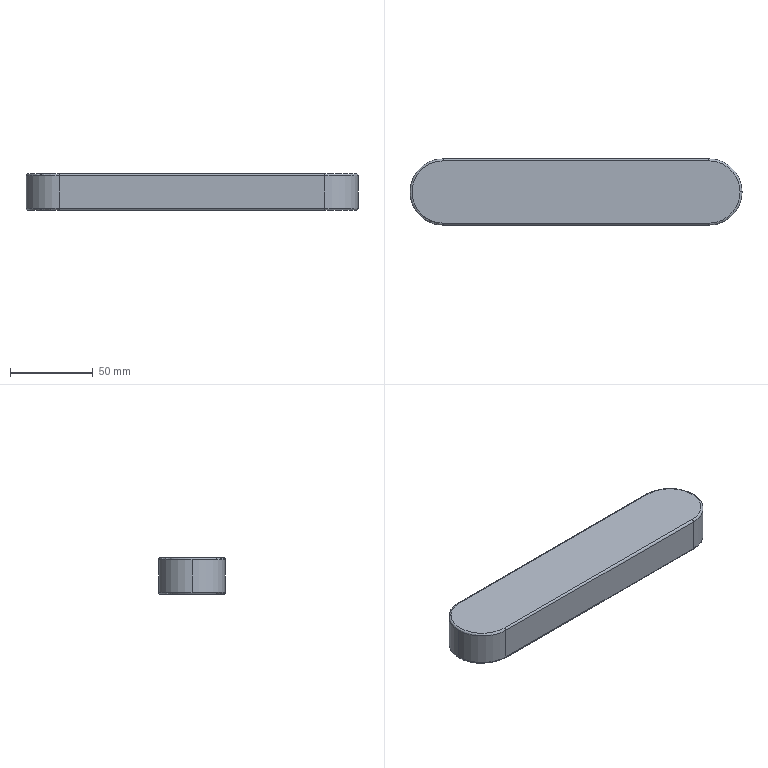Part | SolidWorks | features Extrusion 1, Fillet 1 | 1 solid | 17 faces | box 200 x 40 x 22 mm | volume 168172 mm3 | cylinder 7 | torus 6 | plane 4 | commonest cylinder face diameters 2.4 x4 40 x3
STEP:
#1=CARTESIAN_POINT('',(98.8,0.,0.));
#2=VERTEX_POINT('',#1);
#3=CARTESIAN_POINT('',(80.,-18.8,0.));
#4=VERTEX_POINT('',#3);
#5=CARTESIAN_POINT('',(80.,0.,0.));
#6=DIRECTION('',(0.,0.,-1.));
#7=DIRECTION('',(1.,0.,0.));
#8=AXIS2_PLACEMENT_3D('',#5,#6,#7);
#9=CIRCLE('',#8,18.8);
#10=EDGE_CURVE('',#2,#4,#9,.T.);
#11=ORIENTED_EDGE('',*,*,#10,.F.);
#12=CARTESIAN_POINT('',(100.,0.,1.2));
#13=VERTEX_POINT('',#12);
#14=CARTESIAN_POINT('',(98.8,0.,1.2));
#15=DIRECTION('',(0.,-1.,0.));
#16=DIRECTION('',(0.,0.,-1.));
#17=AXIS2_PLACEMENT_3D('',#14,#15,#16);
#18=CIRCLE('',#17,1.2);
#19=EDGE_CURVE('',#2,#13,#18,.T.);
#20=ORIENTED_EDGE('',*,*,#19,.T.);
#21=CARTESIAN_POINT('',(80.,-20.,1.2));
#22=VERTEX_POINT('',#21);
#23=CARTESIAN_POINT('',(80.,0.,1.2));
#24=DIRECTION('',(0.,0.,1.));
#25=DIRECTION('',(1.,0.,0.));
#26=AXIS2_PLACEMENT_3D('',#23,#24,#25);
#27=CIRCLE('',#26,20.);
#28=EDGE_CURVE('',#22,#13,#27,.T.);
#29=ORIENTED_EDGE('',*,*,#28,.F.);
#30=CARTESIAN_POINT('',(80.,-18.8,1.2));
#31=DIRECTION('',(1.,0.,0.));
#32=DIRECTION('',(0.,0.,-1.));
#33=AXIS2_PLACEMENT_3D('',#30,#31,#32);
#34=CIRCLE('',#33,1.2);
#35=EDGE_CURVE('',#22,#4,#34,.T.);
#36=ORIENTED_EDGE('',*,*,#35,.T.);
#37=EDGE_LOOP('',(#11,#20,#29,#36));
#38=FACE_OUTER_BOUND('',#37,.T.);
#39=CARTESIAN_POINT('',(80.,0.,1.2));
#40=DIRECTION('',(0.,0.,1.));
#41=DIRECTION('',(1.,0.,0.));
#42=AXIS2_PLACEMENT_3D('',#39,#40,#41);
#43=TOROIDAL_SURFACE('',#42,18.8,1.2);
#44=ADVANCED_FACE('',(#38),#43,.T.);
#45=CARTESIAN_POINT('',(100.,0.,20.8));
#46=VERTEX_POINT('',#45);
#47=CARTESIAN_POINT('',(80.,-20.,20.8));
#48=VERTEX_POINT('',#47);
#49=CARTESIAN_POINT('',(80.,0.,20.8));
#50=DIRECTION('',(0.,0.,-1.));
#51=DIRECTION('',(1.,0.,0.));
#52=AXIS2_PLACEMENT_3D('',#49,#50,#51);
#53=CIRCLE('',#52,20.);
#54=EDGE_CURVE('',#46,#48,#53,.T.);
#55=ORIENTED_EDGE('',*,*,#54,.F.);
#56=CARTESIAN_POINT('',(98.8,0.,22.));
#57=VERTEX_POINT('',#56);
#58=CARTESIAN_POINT('',(98.8,0.,20.8));
#59=DIRECTION('',(0.,-1.,0.));
#60=DIRECTION('',(0.,0.,-1.));
#61=AXIS2_PLACEMENT_3D('',#58,#59,#60);
#62=CIRCLE('',#61,1.2);
#63=EDGE_CURVE('',#46,#57,#62,.T.);
#64=ORIENTED_EDGE('',*,*,#63,.T.);
#65=CARTESIAN_POINT('',(80.,-18.8,22.));
#66=VERTEX_POINT('',#65);
#67=CARTESIAN_POINT('',(80.,0.,22.));
#68=DIRECTION('',(0.,0.,1.));
#69=DIRECTION('',(1.,0.,0.));
#70=AXIS2_PLACEMENT_3D('',#67,#68,#69);
#71=CIRCLE('',#70,18.8);
#72=EDGE_CURVE('',#66,#57,#71,.T.);
#73=ORIENTED_EDGE('',*,*,#72,.F.);
#74=CARTESIAN_POINT('',(80.,-18.8,20.8));
#75=DIRECTION('',(1.,0.,0.));
#76=DIRECTION('',(0.,0.,-1.));
#77=AXIS2_PLACEMENT_3D('',#74,#75,#76);
#78=CIRCLE('',#77,1.2);
#79=EDGE_CURVE('',#66,#48,#78,.T.);
#80=ORIENTED_EDGE('',*,*,#79,.T.);
#81=EDGE_LOOP('',(#55,#64,#73,#80));
#82=FACE_OUTER_BOUND('',#81,.T.);
#83=CARTESIAN_POINT('',(80.,0.,20.8));
#84=DIRECTION('',(0.,0.,1.));
#85=DIRECTION('',(1.,0.,0.));
#86=AXIS2_PLACEMENT_3D('',#83,#84,#85);
#87=TOROIDAL_SURFACE('',#86,18.8,1.2);
#88=ADVANCED_FACE('',(#82),#87,.T.);
#89=CARTESIAN_POINT('',(-80.,-20.,20.8));
#90=VERTEX_POINT('',#89);
#91=CARTESIAN_POINT('',(-100.,0.,20.8));
#92=VERTEX_POINT('',#91);
#93=CARTESIAN_POINT('',(-80.,0.,20.8));
#94=DIRECTION('',(0.,0.,-1.));
#95=DIRECTION('',(1.,0.,0.));
#96=AXIS2_PLACEMENT_3D('',#93,#94,#95);
#97=CIRCLE('',#96,20.);
#98=EDGE_CURVE('',#90,#92,#97,.T.);
#99=ORIENTED_EDGE('',*,*,#98,.T.);
#100=CARTESIAN_POINT('',(-100.,0.,1.2));
#101=VERTEX_POINT('',#100);
#102=CARTESIAN_POINT('',(-100.,0.,22.));
#103=DIRECTION('',(0.,0.,-1.));
#104=VECTOR('',#103,1000.);
#105=LINE('',#102,#104);
#106=EDGE_CURVE('',#92,#101,#105,.T.);
#107=ORIENTED_EDGE('',*,*,#106,.T.);
#108=CARTESIAN_POINT('',(-80.,-20.,1.2));
#109=VERTEX_POINT('',#108);
#110=CARTESIAN_POINT('',(-80.,0.,1.2));
#111=DIRECTION('',(0.,0.,1.));
#112=DIRECTION('',(1.,0.,0.));
#113=AXIS2_PLACEMENT_3D('',#110,#111,#112);
#114=CIRCLE('',#113,20.);
#115=EDGE_CURVE('',#101,#109,#114,.T.);
#116=ORIENTED_EDGE('',*,*,#115,.T.);
#117=CARTESIAN_POINT('',(-80.,-20.,22.));
#118=DIRECTION('',(0.,0.,-1.));
#119=VECTOR('',#118,1000.);
#120=LINE('',#117,#119);
#121=EDGE_CURVE('',#90,#109,#120,.T.);
#122=ORIENTED_EDGE('',*,*,#121,.F.);
#123=EDGE_LOOP('',(#99,#107,#116,#122));
#124=FACE_OUTER_BOUND('',#123,.T.);
#125=CARTESIAN_POINT('',(-80.,0.,22.));
#126=DIRECTION('',(0.,0.,-1.));
#127=DIRECTION('',(-1.,0.,0.));
#128=AXIS2_PLACEMENT_3D('',#125,#126,#127);
#129=CYLINDRICAL_SURFACE('',#128,20.);
#130=ADVANCED_FACE('',(#124),#129,.T.);
#131=ORIENTED_EDGE('',*,*,#106,.F.);
#132=CARTESIAN_POINT('',(-80.,20.,20.8));
#133=VERTEX_POINT('',#132);
#134=CARTESIAN_POINT('',(-80.,0.,20.8));
#135=DIRECTION('',(0.,0.,-1.));
#136=DIRECTION('',(1.,0.,0.));
#137=AXIS2_PLACEMENT_3D('',#134,#135,#136);
#138=CIRCLE('',#137,20.);
#139=EDGE_CURVE('',#92,#133,#138,.T.);
#140=ORIENTED_EDGE('',*,*,#139,.T.);
#141=CARTESIAN_POINT('',(-80.,20.,1.2));
#142=VERTEX_POINT('',#141);
#143=CARTESIAN_POINT('',(-80.,20.,22.));
#144=DIRECTION('',(0.,0.,-1.));
#145=VECTOR('',#144,1000.);
#146=LINE('',#143,#145);
#147=EDGE_CURVE('',#133,#142,#146,.T.);
#148=ORIENTED_EDGE('',*,*,#147,.T.);
#149=CARTESIAN_POINT('',(-80.,0.,1.2));
#150=DIRECTION('',(0.,0.,1.));
#151=DIRECTION('',(1.,0.,0.));
#152=AXIS2_PLACEMENT_3D('',#149,#150,#151);
#153=CIRCLE('',#152,20.);
#154=EDGE_CURVE('',#142,#101,#153,.T.);
#155=ORIENTED_EDGE('',*,*,#154,.T.);
#156=EDGE_LOOP('',(#131,#140,#148,#155));
#157=FACE_OUTER_BOUND('',#156,.T.);
#158=CARTESIAN_POINT('',(-80.,0.,22.));
#159=DIRECTION('',(0.,0.,-1.));
#160=DIRECTION('',(-1.,0.,0.));
#161=AXIS2_PLACEMENT_3D('',#158,#159,#160);
#162=CYLINDRICAL_SURFACE('',#161,20.);
#163=ADVANCED_FACE('',(#157),#162,.T.);
#164=CARTESIAN_POINT('',(80.,-20.,22.));
#165=DIRECTION('',(0.,0.,-1.));
#166=VECTOR('',#165,1000.);
#167=LINE('',#164,#166);
#168=EDGE_CURVE('',#48,#22,#167,.T.);
#169=ORIENTED_EDGE('',*,*,#168,.F.);
#170=CARTESIAN_POINT('',(-80.,-20.,20.8));
#171=DIRECTION('',(-1.,0.,0.));
#172=VECTOR('',#171,1000.);
#173=LINE('',#170,#172);
#174=EDGE_CURVE('',#48,#90,#173,.T.);
#175=ORIENTED_EDGE('',*,*,#174,.T.);
#176=ORIENTED_EDGE('',*,*,#121,.T.);
#177=CARTESIAN_POINT('',(-80.,-20.,1.2));
#178=DIRECTION('',(1.,0.,0.));
#179=VECTOR('',#178,1000.);
#180=LINE('',#177,#179);
#181=EDGE_CURVE('',#109,#22,#180,.T.);
#182=ORIENTED_EDGE('',*,*,#181,.T.);
#183=EDGE_LOOP('',(#169,#175,#176,#182));
#184=FACE_OUTER_BOUND('',#183,.T.);
#185=CARTESIAN_POINT('',(-80.,-20.,22.));
#186=DIRECTION('',(0.,1.,0.));
#187=DIRECTION('',(-1.,0.,0.));
#188=AXIS2_PLACEMENT_3D('',#185,#186,#187);
#189=PLANE('',#188);
#190=ADVANCED_FACE('',(#184),#189,.F.);
#191=CARTESIAN_POINT('',(80.,20.,20.8));
#192=VERTEX_POINT('',#191);
#193=CARTESIAN_POINT('',(80.,20.,1.2));
#194=VERTEX_POINT('',#193);
#195=CARTESIAN_POINT('',(80.,20.,22.));
#196=DIRECTION('',(0.,0.,-1.));
#197=VECTOR('',#196,1000.);
#198=LINE('',#195,#197);
#199=EDGE_CURVE('',#192,#194,#198,.T.);
#200=ORIENTED_EDGE('',*,*,#199,.F.);
#201=CARTESIAN_POINT('',(80.,0.,20.8));
#202=DIRECTION('',(0.,0.,-1.));
#203=DIRECTION('',(1.,0.,0.));
#204=AXIS2_PLACEMENT_3D('',#201,#202,#203);
#205=CIRCLE('',#204,20.);
#206=EDGE_CURVE('',#192,#46,#205,.T.);
#207=ORIENTED_EDGE('',*,*,#206,.T.);
#208=ORIENTED_EDGE('',*,*,#54,.T.);
#209=ORIENTED_EDGE('',*,*,#168,.T.);
#210=ORIENTED_EDGE('',*,*,#28,.T.);
#211=CARTESIAN_POINT('',(80.,0.,1.2));
#212=DIRECTION('',(0.,0.,1.));
#213=DIRECTION('',(1.,0.,0.));
#214=AXIS2_PLACEMENT_3D('',#211,#212,#213);
#215=CIRCLE('',#214,20.);
#216=EDGE_CURVE('',#13,#194,#215,.T.);
#217=ORIENTED_EDGE('',*,*,#216,.T.);
#218=EDGE_LOOP('',(#200,#207,#208,#209,#210,#217));
#219=FACE_OUTER_BOUND('',#218,.T.);
#220=CARTESIAN_POINT('',(80.,0.,22.));
#221=DIRECTION('',(0.,0.,-1.));
#222=DIRECTION('',(-1.,0.,0.));
#223=AXIS2_PLACEMENT_3D('',#220,#221,#222);
#224=CYLINDRICAL_SURFACE('',#223,20.);
#225=ADVANCED_FACE('',(#219),#224,.T.);
#226=ORIENTED_EDGE('',*,*,#147,.F.);
#227=CARTESIAN_POINT('',(80.,20.,20.8));
#228=DIRECTION('',(1.,0.,0.));
#229=VECTOR('',#228,1000.);
#230=LINE('',#227,#229);
#231=EDGE_CURVE('',#133,#192,#230,.T.);
#232=ORIENTED_EDGE('',*,*,#231,.T.);
#233=ORIENTED_EDGE('',*,*,#199,.T.);
#234=CARTESIAN_POINT('',(-80.,20.,1.2));
#235=DIRECTION('',(-1.,0.,0.));
#236=VECTOR('',#235,1000.);
#237=LINE('',#234,#236);
#238=EDGE_CURVE('',#194,#142,#237,.T.);
#239=ORIENTED_EDGE('',*,*,#238,.T.);
#240=EDGE_LOOP('',(#226,#232,#233,#239));
#241=FACE_OUTER_BOUND('',#240,.T.);
#242=CARTESIAN_POINT('',(-80.,20.,22.));
#243=DIRECTION('',(0.,-1.,0.));
#244=DIRECTION('',(1.,0.,0.));
#245=AXIS2_PLACEMENT_3D('',#242,#243,#244);
#246=PLANE('',#245);
#247=ADVANCED_FACE('',(#241),#246,.F.);
#248=CARTESIAN_POINT('',(-80.,-18.8,22.));
#249=VERTEX_POINT('',#248);
#250=CARTESIAN_POINT('',(80.,-18.8,22.));
#251=DIRECTION('',(1.,0.,0.));
#252=VECTOR('',#251,1000.);
#253=LINE('',#250,#252);
#254=EDGE_CURVE('',#249,#66,#253,.T.);
#255=ORIENTED_EDGE('',*,*,#254,.T.);
#256=ORIENTED_EDGE('',*,*,#72,.T.);
#257=CARTESIAN_POINT('',(80.,18.8,22.));
#258=VERTEX_POINT('',#257);
#259=CARTESIAN_POINT('',(80.,0.,22.));
#260=DIRECTION('',(0.,0.,1.));
#261=DIRECTION('',(1.,0.,0.));
#262=AXIS2_PLACEMENT_3D('',#259,#260,#261);
#263=CIRCLE('',#262,18.8);
#264=EDGE_CURVE('',#57,#258,#263,.T.);
#265=ORIENTED_EDGE('',*,*,#264,.T.);
#266=CARTESIAN_POINT('',(-80.,18.8,22.));
#267=VERTEX_POINT('',#266);
#268=CARTESIAN_POINT('',(-80.,18.8,22.));
#269=DIRECTION('',(-1.,0.,0.));
#270=VECTOR('',#269,1000.);
#271=LINE('',#268,#270);
#272=EDGE_CURVE('',#258,#267,#271,.T.);
#273=ORIENTED_EDGE('',*,*,#272,.T.);
#274=CARTESIAN_POINT('',(-80.,0.,22.));
#275=DIRECTION('',(0.,0.,1.));
#276=DIRECTION('',(1.,0.,0.));
#277=AXIS2_PLACEMENT_3D('',#274,#275,#276);
#278=CIRCLE('',#277,18.8);
#279=EDGE_CURVE('',#267,#249,#278,.T.);
#280=ORIENTED_EDGE('',*,*,#279,.T.);
#281=EDGE_LOOP('',(#255,#256,#265,#273,#280));
#282=FACE_OUTER_BOUND('',#281,.T.);
#283=CARTESIAN_POINT('',(-80.,0.,22.));
#284=DIRECTION('',(0.,0.,1.));
#285=DIRECTION('',(1.,0.,0.));
#286=AXIS2_PLACEMENT_3D('',#283,#284,#285);
#287=PLANE('',#286);
#288=ADVANCED_FACE('',(#282),#287,.T.);
#289=CARTESIAN_POINT('',(-80.,18.8,0.));
#290=VERTEX_POINT('',#289);
#291=CARTESIAN_POINT('',(80.,18.8,0.));
#292=VERTEX_POINT('',#291);
#293=CARTESIAN_POINT('',(-80.,18.8,0.));
#294=DIRECTION('',(1.,0.,0.));
#295=VECTOR('',#294,1000.);
#296=LINE('',#293,#295);
#297=EDGE_CURVE('',#290,#292,#296,.T.);
#298=ORIENTED_EDGE('',*,*,#297,.T.);
#299=CARTESIAN_POINT('',(80.,0.,0.));
#300=DIRECTION('',(0.,0.,-1.));
#301=DIRECTION('',(1.,0.,0.));
#302=AXIS2_PLACEMENT_3D('',#299,#300,#301);
#303=CIRCLE('',#302,18.8);
#304=EDGE_CURVE('',#292,#2,#303,.T.);
#305=ORIENTED_EDGE('',*,*,#304,.T.);
#306=ORIENTED_EDGE('',*,*,#10,.T.);
#307=CARTESIAN_POINT('',(-80.,-18.8,0.));
#308=VERTEX_POINT('',#307);
#309=CARTESIAN_POINT('',(-80.,-18.8,0.));
#310=DIRECTION('',(-1.,0.,0.));
#311=VECTOR('',#310,1000.);
#312=LINE('',#309,#311);
#313=EDGE_CURVE('',#4,#308,#312,.T.);
#314=ORIENTED_EDGE('',*,*,#313,.T.);
#315=CARTESIAN_POINT('',(-80.,0.,0.));
#316=DIRECTION('',(0.,0.,-1.));
#317=DIRECTION('',(1.,0.,0.));
#318=AXIS2_PLACEMENT_3D('',#315,#316,#317);
#319=CIRCLE('',#318,18.8);
#320=EDGE_CURVE('',#308,#290,#319,.T.);
#321=ORIENTED_EDGE('',*,*,#320,.T.);
#322=EDGE_LOOP('',(#298,#305,#306,#314,#321));
#323=FACE_OUTER_BOUND('',#322,.T.);
#324=CARTESIAN_POINT('',(-80.,0.,0.));
#325=DIRECTION('',(0.,0.,1.));
#326=DIRECTION('',(1.,0.,0.));
#327=AXIS2_PLACEMENT_3D('',#324,#325,#326);
#328=PLANE('',#327);
#329=ADVANCED_FACE('',(#323),#328,.F.);
#330=CARTESIAN_POINT('',(-80.,18.8,20.8));
#331=DIRECTION('',(1.,0.,0.));
#332=DIRECTION('',(0.,0.,-1.));
#333=AXIS2_PLACEMENT_3D('',#330,#331,#332);
#334=CIRCLE('',#333,1.2);
#335=EDGE_CURVE('',#133,#267,#334,.T.);
#336=ORIENTED_EDGE('',*,*,#335,.F.);
#337=ORIENTED_EDGE('',*,*,#139,.F.);
#338=ORIENTED_EDGE('',*,*,#98,.F.);
#339=CARTESIAN_POINT('',(-80.,-18.8,20.8));
#340=DIRECTION('',(1.,0.,0.));
#341=DIRECTION('',(0.,0.,-1.));
#342=AXIS2_PLACEMENT_3D('',#339,#340,#341);
#343=CIRCLE('',#342,1.2);
#344=EDGE_CURVE('',#249,#90,#343,.T.);
#345=ORIENTED_EDGE('',*,*,#344,.F.);
#346=ORIENTED_EDGE('',*,*,#279,.F.);
#347=EDGE_LOOP('',(#336,#337,#338,#345,#346));
#348=FACE_OUTER_BOUND('',#347,.T.);
#349=CARTESIAN_POINT('',(-80.,0.,20.8));
#350=DIRECTION('',(0.,0.,1.));
#351=DIRECTION('',(1.,0.,0.));
#352=AXIS2_PLACEMENT_3D('',#349,#350,#351);
#353=TOROIDAL_SURFACE('',#352,18.8,1.2);
#354=ADVANCED_FACE('',(#348),#353,.T.);
#355=ORIENTED_EDGE('',*,*,#344,.T.);
#356=ORIENTED_EDGE('',*,*,#174,.F.);
#357=ORIENTED_EDGE('',*,*,#79,.F.);
#358=ORIENTED_EDGE('',*,*,#254,.F.);
#359=EDGE_LOOP('',(#355,#356,#357,#358));
#360=FACE_OUTER_BOUND('',#359,.T.);
#361=CARTESIAN_POINT('',(-80.,-18.8,20.8));
#362=DIRECTION('',(-1.,0.,0.));
#363=DIRECTION('',(0.,-1.,0.));
#364=AXIS2_PLACEMENT_3D('',#361,#362,#363);
#365=CYLINDRICAL_SURFACE('',#364,1.2);
#366=ADVANCED_FACE('',(#360),#365,.T.);
#367=ORIENTED_EDGE('',*,*,#335,.T.);
#368=ORIENTED_EDGE('',*,*,#272,.F.);
#369=CARTESIAN_POINT('',(80.,18.8,20.8));
#370=DIRECTION('',(1.,0.,0.));
#371=DIRECTION('',(0.,0.,-1.));
#372=AXIS2_PLACEMENT_3D('',#369,#370,#371);
#373=CIRCLE('',#372,1.2);
#374=EDGE_CURVE('',#192,#258,#373,.T.);
#375=ORIENTED_EDGE('',*,*,#374,.F.);
#376=ORIENTED_EDGE('',*,*,#231,.F.);
#377=EDGE_LOOP('',(#367,#368,#375,#376));
#378=FACE_OUTER_BOUND('',#377,.T.);
#379=CARTESIAN_POINT('',(-80.,18.8,20.8));
#380=DIRECTION('',(1.,0.,0.));
#381=DIRECTION('',(0.,1.,0.));
#382=AXIS2_PLACEMENT_3D('',#379,#380,#381);
#383=CYLINDRICAL_SURFACE('',#382,1.2);
#384=ADVANCED_FACE('',(#378),#383,.T.);
#385=ORIENTED_EDGE('',*,*,#63,.F.);
#386=ORIENTED_EDGE('',*,*,#206,.F.);
#387=ORIENTED_EDGE('',*,*,#374,.T.);
#388=ORIENTED_EDGE('',*,*,#264,.F.);
#389=EDGE_LOOP('',(#385,#386,#387,#388));
#390=FACE_OUTER_BOUND('',#389,.T.);
#391=CARTESIAN_POINT('',(80.,0.,20.8));
#392=DIRECTION('',(0.,0.,1.));
#393=DIRECTION('',(1.,0.,0.));
#394=AXIS2_PLACEMENT_3D('',#391,#392,#393);
#395=TOROIDAL_SURFACE('',#394,18.8,1.2);
#396=ADVANCED_FACE('',(#390),#395,.T.);
#397=CARTESIAN_POINT('',(-80.,18.8,1.2));
#398=DIRECTION('',(1.,0.,0.));
#399=DIRECTION('',(0.,0.,-1.));
#400=AXIS2_PLACEMENT_3D('',#397,#398,#399);
#401=CIRCLE('',#400,1.2);
#402=EDGE_CURVE('',#290,#142,#401,.T.);
#403=ORIENTED_EDGE('',*,*,#402,.F.);
#404=ORIENTED_EDGE('',*,*,#320,.F.);
#405=CARTESIAN_POINT('',(-80.,-18.8,1.2));
#406=DIRECTION('',(1.,0.,0.));
#407=DIRECTION('',(0.,0.,-1.));
#408=AXIS2_PLACEMENT_3D('',#405,#406,#407);
#409=CIRCLE('',#408,1.2);
#410=EDGE_CURVE('',#109,#308,#409,.T.);
#411=ORIENTED_EDGE('',*,*,#410,.F.);
#412=ORIENTED_EDGE('',*,*,#115,.F.);
#413=ORIENTED_EDGE('',*,*,#154,.F.);
#414=EDGE_LOOP('',(#403,#404,#411,#412,#413));
#415=FACE_OUTER_BOUND('',#414,.T.);
#416=CARTESIAN_POINT('',(-80.,0.,1.2));
#417=DIRECTION('',(0.,0.,1.));
#418=DIRECTION('',(1.,0.,0.));
#419=AXIS2_PLACEMENT_3D('',#416,#417,#418);
#420=TOROIDAL_SURFACE('',#419,18.8,1.2);
#421=ADVANCED_FACE('',(#415),#420,.T.);
#422=ORIENTED_EDGE('',*,*,#410,.T.);
#423=ORIENTED_EDGE('',*,*,#313,.F.);
#424=ORIENTED_EDGE('',*,*,#35,.F.);
#425=ORIENTED_EDGE('',*,*,#181,.F.);
#426=EDGE_LOOP('',(#422,#423,#424,#425));
#427=FACE_OUTER_BOUND('',#426,.T.);
#428=CARTESIAN_POINT('',(-80.,-18.8,1.2));
#429=DIRECTION('',(1.,0.,0.));
#430=DIRECTION('',(0.,1.,0.));
#431=AXIS2_PLACEMENT_3D('',#428,#429,#430);
#432=CYLINDRICAL_SURFACE('',#431,1.2);
#433=ADVANCED_FACE('',(#427),#432,.T.);
#434=ORIENTED_EDGE('',*,*,#402,.T.);
#435=ORIENTED_EDGE('',*,*,#238,.F.);
#436=CARTESIAN_POINT('',(80.,18.8,1.2));
#437=DIRECTION('',(1.,0.,0.));
#438=DIRECTION('',(0.,0.,-1.));
#439=AXIS2_PLACEMENT_3D('',#436,#437,#438);
#440=CIRCLE('',#439,1.2);
#441=EDGE_CURVE('',#292,#194,#440,.T.);
#442=ORIENTED_EDGE('',*,*,#441,.F.);
#443=ORIENTED_EDGE('',*,*,#297,.F.);
#444=EDGE_LOOP('',(#434,#435,#442,#443));
#445=FACE_OUTER_BOUND('',#444,.T.);
#446=CARTESIAN_POINT('',(-80.,18.8,1.2));
#447=DIRECTION('',(-1.,0.,0.));
#448=DIRECTION('',(0.,-1.,0.));
#449=AXIS2_PLACEMENT_3D('',#446,#447,#448);
#450=CYLINDRICAL_SURFACE('',#449,1.2);
#451=ADVANCED_FACE('',(#445),#450,.T.);
#452=ORIENTED_EDGE('',*,*,#19,.F.);
#453=ORIENTED_EDGE('',*,*,#304,.F.);
#454=ORIENTED_EDGE('',*,*,#441,.T.);
#455=ORIENTED_EDGE('',*,*,#216,.F.);
#456=EDGE_LOOP('',(#452,#453,#454,#455));
#457=FACE_OUTER_BOUND('',#456,.T.);
#458=CARTESIAN_POINT('',(80.,0.,1.2));
#459=DIRECTION('',(0.,0.,1.));
#460=DIRECTION('',(1.,0.,0.));
#461=AXIS2_PLACEMENT_3D('',#458,#459,#460);
#462=TOROIDAL_SURFACE('',#461,18.8,1.2);
#463=ADVANCED_FACE('',(#457),#462,.T.);
#464=CLOSED_SHELL('',(#44,#88,#130,#163,#190,#225,#247,#288,#329,#354,#366,#384,#396,#421,#433,#451,#463));
#465=MANIFOLD_SOLID_BREP('',#464);
#466=CARTESIAN_POINT('',(0.,0.,0.));
#467=DIRECTION('',(0.,0.,1.));
#468=DIRECTION('',(1.,0.,0.));
#469=AXIS2_PLACEMENT_3D('',#466,#467,#468);
#470=(LENGTH_UNIT()NAMED_UNIT(*)SI_UNIT(.MILLI.,.METRE.));
#471=UNCERTAINTY_MEASURE_WITH_UNIT(LENGTH_MEASURE(0.00001),#470,'','');
#472=(NAMED_UNIT(*)PLANE_ANGLE_UNIT()SI_UNIT($,.RADIAN.));
#473=(NAMED_UNIT(*)SI_UNIT($,.STERADIAN.)SOLID_ANGLE_UNIT());
#474=(GEOMETRIC_REPRESENTATION_CONTEXT(3)GLOBAL_UNCERTAINTY_ASSIGNED_CONTEXT((#471))GLOBAL_UNIT_ASSIGNED_CONTEXT((#470,#472,#473))REPRESENTATION_CONTEXT('',''));
#475=ADVANCED_BREP_SHAPE_REPRESENTATION('',(#465,#469),#474);